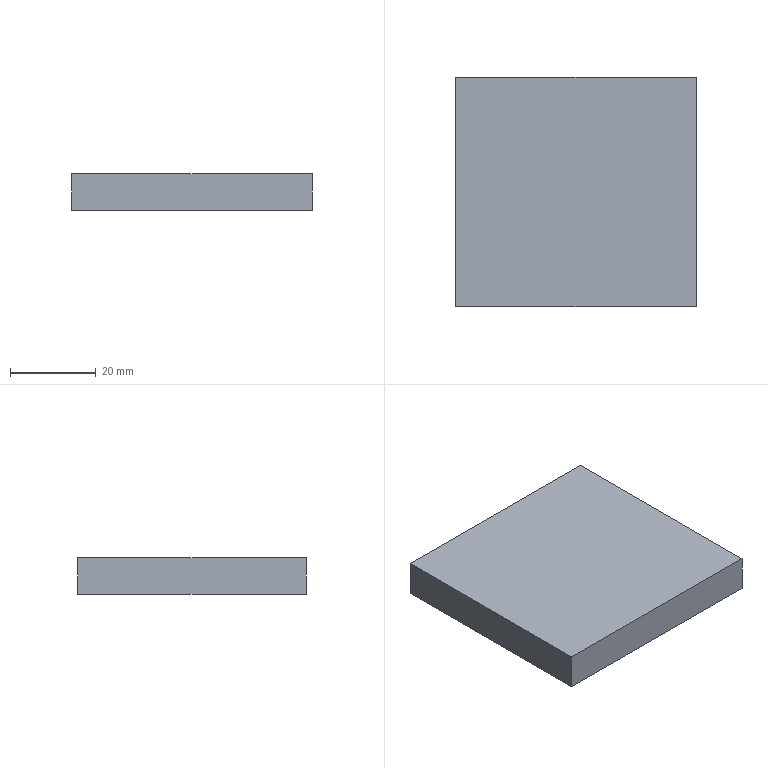NC program | NX | posted with a generic post | part box 56 x 53.3 x 8.5 mm
Lines 1 to 34 of 5023:
N10 G17 G21 G94 G90
(FLOOR_WALL_COPY_COPY , TOOL : D80)
N12 T19 M6
N14 G54
N16 G17 G0 G90 X-68. Y0. S6500 M3
N18 G43 Z30. H19
N20 Z4.
N22 G94 G1 Z1. F1500.
N24 X-63.
N26 X63.
N28 X68.
N30 Z4.
N32 G0 Z30.
N34 X-68.
N36 Z3.5
N38 G1 Z0.5
N40 X-63.
N42 X63.
N44 X68.
N46 Z3.5
N48 G0 Z30.
N50 X-68.
N52 Z3.
N54 G1 Z0.
N56 X-63.
N58 X63.
N60 X68.
N62 Z3.
N64 G0 Z30.
N66 M5